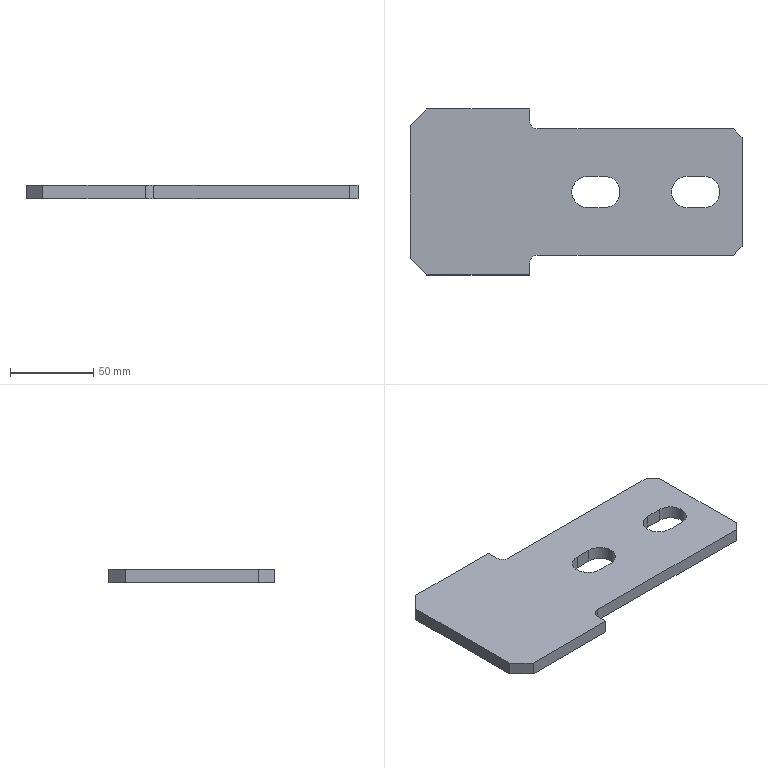Part | STEP file | 立柱腹Plate筋Plate-194×150-12 | 1 solid | 26 faces | box 200 x 100 x 8 mm | volume 126933 mm3 | plane 18 | cylinder 8 | commonest cylinder face diameters 19 x6 10 x2